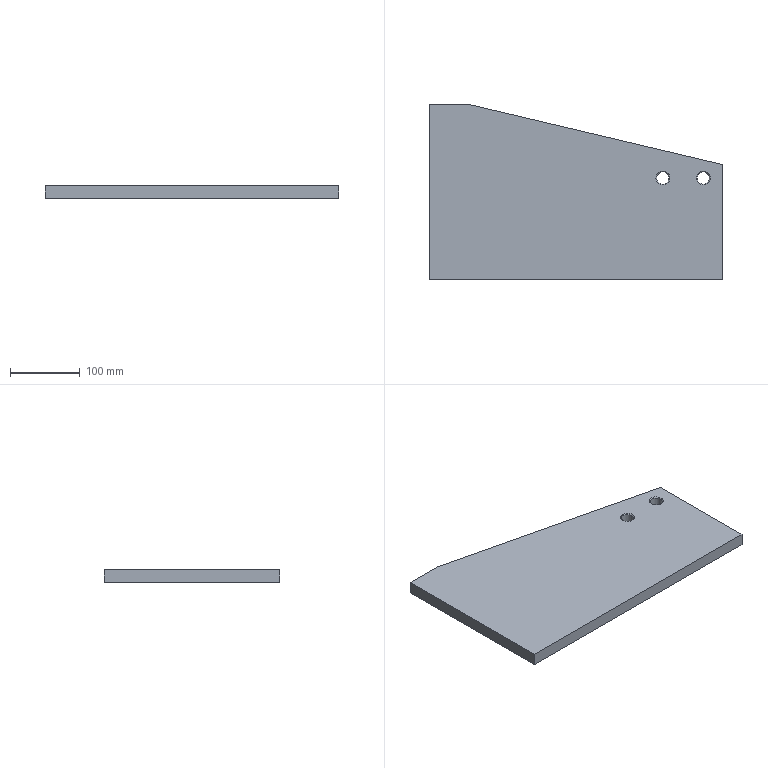Part | NX | features BREP 1 | 1 solid | 13 faces | box 421 x 252 x 18 mm | volume 1615279 mm3 | plane 7 | cone 4 | cylinder 2 | commonest cylinder face diameters 17.5 x2
STEP:
#1=CARTESIAN_POINT('',(-319.,-146.,-144.));
#2=VERTEX_POINT('',#1);
#3=CARTESIAN_POINT('',(-319.,106.,-144.));
#4=VERTEX_POINT('',#3);
#5=CARTESIAN_POINT('',(-319.,-146.,-144.));
#6=DIRECTION('',(0.,1.,0.));
#7=VECTOR('',#6,1000.);
#8=LINE('',#5,#7);
#9=EDGE_CURVE('',#2,#4,#8,.T.);
#10=ORIENTED_EDGE('',*,*,#9,.F.);
#11=CARTESIAN_POINT('',(-319.,-146.,-126.));
#12=VERTEX_POINT('',#11);
#13=CARTESIAN_POINT('',(-319.,-146.,-126.));
#14=DIRECTION('',(0.,0.,-1.));
#15=VECTOR('',#14,1000.);
#16=LINE('',#13,#15);
#17=EDGE_CURVE('',#12,#2,#16,.T.);
#18=ORIENTED_EDGE('',*,*,#17,.F.);
#19=CARTESIAN_POINT('',(-319.,106.,-126.));
#20=VERTEX_POINT('',#19);
#21=CARTESIAN_POINT('',(-319.,-146.,-126.));
#22=DIRECTION('',(0.,1.,0.));
#23=VECTOR('',#22,1000.);
#24=LINE('',#21,#23);
#25=EDGE_CURVE('',#12,#20,#24,.T.);
#26=ORIENTED_EDGE('',*,*,#25,.T.);
#27=CARTESIAN_POINT('',(-319.,106.,-126.));
#28=DIRECTION('',(0.,0.,-1.));
#29=VECTOR('',#28,1000.);
#30=LINE('',#27,#29);
#31=EDGE_CURVE('',#20,#4,#30,.T.);
#32=ORIENTED_EDGE('',*,*,#31,.T.);
#33=EDGE_LOOP('',(#10,#18,#26,#32));
#34=FACE_BOUND('',#33,.T.);
#35=CARTESIAN_POINT('',(-319.,-146.,-126.));
#36=DIRECTION('',(-1.,0.,0.));
#37=DIRECTION('',(0.,-1.,0.));
#38=AXIS2_PLACEMENT_3D('',#35,#36,#37);
#39=PLANE('',#38);
#40=ADVANCED_FACE('',(#34),#39,.T.);
#41=CARTESIAN_POINT('',(-264.,106.,-144.));
#42=VERTEX_POINT('',#41);
#43=CARTESIAN_POINT('',(-319.,106.,-144.));
#44=DIRECTION('',(1.,0.,0.));
#45=VECTOR('',#44,1000.);
#46=LINE('',#43,#45);
#47=EDGE_CURVE('',#4,#42,#46,.T.);
#48=ORIENTED_EDGE('',*,*,#47,.F.);
#49=ORIENTED_EDGE('',*,*,#31,.F.);
#50=CARTESIAN_POINT('',(-264.,106.,-126.));
#51=VERTEX_POINT('',#50);
#52=CARTESIAN_POINT('',(-319.,106.,-126.));
#53=DIRECTION('',(1.,0.,0.));
#54=VECTOR('',#53,1000.);
#55=LINE('',#52,#54);
#56=EDGE_CURVE('',#20,#51,#55,.T.);
#57=ORIENTED_EDGE('',*,*,#56,.T.);
#58=CARTESIAN_POINT('',(-264.,106.,-126.));
#59=DIRECTION('',(0.,0.,-1.));
#60=VECTOR('',#59,1000.);
#61=LINE('',#58,#60);
#62=EDGE_CURVE('',#51,#42,#61,.T.);
#63=ORIENTED_EDGE('',*,*,#62,.T.);
#64=EDGE_LOOP('',(#48,#49,#57,#63));
#65=FACE_BOUND('',#64,.T.);
#66=CARTESIAN_POINT('',(-319.,106.,-126.));
#67=DIRECTION('',(0.,1.,0.));
#68=DIRECTION('',(-1.,0.,0.));
#69=AXIS2_PLACEMENT_3D('',#66,#67,#68);
#70=PLANE('',#69);
#71=ADVANCED_FACE('',(#65),#70,.T.);
#72=CARTESIAN_POINT('',(102.,19.316,-144.));
#73=VERTEX_POINT('',#72);
#74=CARTESIAN_POINT('',(-264.,106.,-144.));
#75=DIRECTION('',(0.9731,-0.2305,0.));
#76=VECTOR('',#75,1000.);
#77=LINE('',#74,#76);
#78=EDGE_CURVE('',#42,#73,#77,.T.);
#79=ORIENTED_EDGE('',*,*,#78,.F.);
#80=ORIENTED_EDGE('',*,*,#62,.F.);
#81=CARTESIAN_POINT('',(102.,19.316,-126.));
#82=VERTEX_POINT('',#81);
#83=CARTESIAN_POINT('',(-264.,106.,-126.));
#84=DIRECTION('',(0.9731,-0.2305,0.));
#85=VECTOR('',#84,1000.);
#86=LINE('',#83,#85);
#87=EDGE_CURVE('',#51,#82,#86,.T.);
#88=ORIENTED_EDGE('',*,*,#87,.T.);
#89=CARTESIAN_POINT('',(102.,19.316,-126.));
#90=DIRECTION('',(0.,0.,-1.));
#91=VECTOR('',#90,1000.);
#92=LINE('',#89,#91);
#93=EDGE_CURVE('',#82,#73,#92,.T.);
#94=ORIENTED_EDGE('',*,*,#93,.T.);
#95=EDGE_LOOP('',(#79,#80,#88,#94));
#96=FACE_BOUND('',#95,.T.);
#97=CARTESIAN_POINT('',(-264.,106.,-126.));
#98=DIRECTION('',(0.2305,0.9731,0.));
#99=DIRECTION('',(-0.9731,0.2305,0.));
#100=AXIS2_PLACEMENT_3D('',#97,#98,#99);
#101=PLANE('',#100);
#102=ADVANCED_FACE('',(#96),#101,.T.);
#103=CARTESIAN_POINT('',(102.,-146.,-144.));
#104=VERTEX_POINT('',#103);
#105=CARTESIAN_POINT('',(102.,19.316,-144.));
#106=DIRECTION('',(0.,-1.,0.));
#107=VECTOR('',#106,1000.);
#108=LINE('',#105,#107);
#109=EDGE_CURVE('',#73,#104,#108,.T.);
#110=ORIENTED_EDGE('',*,*,#109,.F.);
#111=ORIENTED_EDGE('',*,*,#93,.F.);
#112=CARTESIAN_POINT('',(102.,-146.,-126.));
#113=VERTEX_POINT('',#112);
#114=CARTESIAN_POINT('',(102.,19.316,-126.));
#115=DIRECTION('',(0.,-1.,0.));
#116=VECTOR('',#115,1000.);
#117=LINE('',#114,#116);
#118=EDGE_CURVE('',#82,#113,#117,.T.);
#119=ORIENTED_EDGE('',*,*,#118,.T.);
#120=CARTESIAN_POINT('',(102.,-146.,-126.));
#121=DIRECTION('',(0.,0.,-1.));
#122=VECTOR('',#121,1000.);
#123=LINE('',#120,#122);
#124=EDGE_CURVE('',#113,#104,#123,.T.);
#125=ORIENTED_EDGE('',*,*,#124,.T.);
#126=EDGE_LOOP('',(#110,#111,#119,#125));
#127=FACE_BOUND('',#126,.T.);
#128=CARTESIAN_POINT('',(102.,19.316,-126.));
#129=DIRECTION('',(1.,0.,0.));
#130=DIRECTION('',(0.,1.,0.));
#131=AXIS2_PLACEMENT_3D('',#128,#129,#130);
#132=PLANE('',#131);
#133=ADVANCED_FACE('',(#127),#132,.T.);
#134=CARTESIAN_POINT('',(102.,-146.,-144.));
#135=DIRECTION('',(-1.,0.,0.));
#136=VECTOR('',#135,1000.);
#137=LINE('',#134,#136);
#138=EDGE_CURVE('',#104,#2,#137,.T.);
#139=ORIENTED_EDGE('',*,*,#138,.F.);
#140=ORIENTED_EDGE('',*,*,#124,.F.);
#141=CARTESIAN_POINT('',(102.,-146.,-126.));
#142=DIRECTION('',(-1.,0.,0.));
#143=VECTOR('',#142,1000.);
#144=LINE('',#141,#143);
#145=EDGE_CURVE('',#113,#12,#144,.T.);
#146=ORIENTED_EDGE('',*,*,#145,.T.);
#147=ORIENTED_EDGE('',*,*,#17,.T.);
#148=EDGE_LOOP('',(#139,#140,#146,#147));
#149=FACE_BOUND('',#148,.T.);
#150=CARTESIAN_POINT('',(102.,-146.,-126.));
#151=DIRECTION('',(0.,-1.,0.));
#152=DIRECTION('',(1.,0.,0.));
#153=AXIS2_PLACEMENT_3D('',#150,#151,#152);
#154=PLANE('',#153);
#155=ADVANCED_FACE('',(#149),#154,.T.);
#156=CARTESIAN_POINT('',(6.,0.,-126.));
#157=VERTEX_POINT('',#156);
#158=CARTESIAN_POINT('',(16.,0.,-126.));
#159=DIRECTION('',(0.,0.,-1.));
#160=DIRECTION('',(-1.,0.,0.));
#161=AXIS2_PLACEMENT_3D('',#158,#159,#160);
#162=CIRCLE('',#161,10.);
#163=EDGE_CURVE('',#157,#157,#162,.T.);
#164=ORIENTED_EDGE('',*,*,#163,.T.);
#165=EDGE_LOOP('',(#164));
#166=FACE_BOUND('',#165,.T.);
#167=CARTESIAN_POINT('',(64.,0.,-126.));
#168=VERTEX_POINT('',#167);
#169=CARTESIAN_POINT('',(74.,0.,-126.));
#170=DIRECTION('',(0.,0.,-1.));
#171=DIRECTION('',(-1.,0.,0.));
#172=AXIS2_PLACEMENT_3D('',#169,#170,#171);
#173=CIRCLE('',#172,10.);
#174=EDGE_CURVE('',#168,#168,#173,.T.);
#175=ORIENTED_EDGE('',*,*,#174,.T.);
#176=EDGE_LOOP('',(#175));
#177=FACE_BOUND('',#176,.T.);
#178=ORIENTED_EDGE('',*,*,#25,.F.);
#179=ORIENTED_EDGE('',*,*,#145,.F.);
#180=ORIENTED_EDGE('',*,*,#118,.F.);
#181=ORIENTED_EDGE('',*,*,#87,.F.);
#182=ORIENTED_EDGE('',*,*,#56,.F.);
#183=EDGE_LOOP('',(#178,#179,#180,#181,#182));
#184=FACE_BOUND('',#183,.T.);
#185=CARTESIAN_POINT('',(0.,0.,-126.));
#186=DIRECTION('',(0.,0.,-1.));
#187=DIRECTION('',(-1.,0.,0.));
#188=AXIS2_PLACEMENT_3D('',#185,#186,#187);
#189=PLANE('',#188);
#190=ADVANCED_FACE('',(#166,#177,#184),#189,.F.);
#191=CARTESIAN_POINT('',(6.,0.,-144.));
#192=VERTEX_POINT('',#191);
#193=CARTESIAN_POINT('',(16.,0.,-144.));
#194=DIRECTION('',(0.,0.,-1.));
#195=DIRECTION('',(-1.,0.,0.));
#196=AXIS2_PLACEMENT_3D('',#193,#194,#195);
#197=CIRCLE('',#196,10.);
#198=EDGE_CURVE('',#192,#192,#197,.F.);
#199=ORIENTED_EDGE('',*,*,#198,.T.);
#200=EDGE_LOOP('',(#199));
#201=FACE_BOUND('',#200,.T.);
#202=CARTESIAN_POINT('',(64.,0.,-144.));
#203=VERTEX_POINT('',#202);
#204=CARTESIAN_POINT('',(74.,0.,-144.));
#205=DIRECTION('',(0.,0.,-1.));
#206=DIRECTION('',(-1.,0.,0.));
#207=AXIS2_PLACEMENT_3D('',#204,#205,#206);
#208=CIRCLE('',#207,10.);
#209=EDGE_CURVE('',#203,#203,#208,.F.);
#210=ORIENTED_EDGE('',*,*,#209,.T.);
#211=EDGE_LOOP('',(#210));
#212=FACE_BOUND('',#211,.T.);
#213=ORIENTED_EDGE('',*,*,#9,.T.);
#214=ORIENTED_EDGE('',*,*,#47,.T.);
#215=ORIENTED_EDGE('',*,*,#78,.T.);
#216=ORIENTED_EDGE('',*,*,#109,.T.);
#217=ORIENTED_EDGE('',*,*,#138,.T.);
#218=EDGE_LOOP('',(#213,#214,#215,#216,#217));
#219=FACE_BOUND('',#218,.T.);
#220=CARTESIAN_POINT('',(0.,0.,-144.));
#221=DIRECTION('',(0.,0.,-1.));
#222=DIRECTION('',(-1.,0.,0.));
#223=AXIS2_PLACEMENT_3D('',#220,#221,#222);
#224=PLANE('',#223);
#225=ADVANCED_FACE('',(#201,#212,#219),#224,.T.);
#226=CARTESIAN_POINT('',(65.25,0.,-127.25));
#227=VERTEX_POINT('',#226);
#228=CARTESIAN_POINT('',(74.,0.,-127.25));
#229=DIRECTION('',(0.,0.,-1.));
#230=DIRECTION('',(-1.,0.,0.));
#231=AXIS2_PLACEMENT_3D('',#228,#229,#230);
#232=CIRCLE('',#231,8.75);
#233=EDGE_CURVE('',#227,#227,#232,.F.);
#234=ORIENTED_EDGE('',*,*,#233,.T.);
#235=EDGE_LOOP('',(#234));
#236=FACE_BOUND('',#235,.T.);
#237=CARTESIAN_POINT('',(65.25,0.,-142.75));
#238=VERTEX_POINT('',#237);
#239=CARTESIAN_POINT('',(74.,0.,-142.75));
#240=DIRECTION('',(0.,0.,-1.));
#241=DIRECTION('',(-1.,0.,0.));
#242=AXIS2_PLACEMENT_3D('',#239,#240,#241);
#243=CIRCLE('',#242,8.75);
#244=EDGE_CURVE('',#238,#238,#243,.T.);
#245=ORIENTED_EDGE('',*,*,#244,.T.);
#246=EDGE_LOOP('',(#245));
#247=FACE_BOUND('',#246,.T.);
#248=CARTESIAN_POINT('',(74.,0.,-144.));
#249=DIRECTION('',(0.,0.,1.));
#250=DIRECTION('',(1.,0.,0.));
#251=AXIS2_PLACEMENT_3D('',#248,#249,#250);
#252=CYLINDRICAL_SURFACE('',#251,8.75);
#253=ADVANCED_FACE('',(#236,#247),#252,.F.);
#254=ORIENTED_EDGE('',*,*,#244,.F.);
#255=EDGE_LOOP('',(#254));
#256=FACE_BOUND('',#255,.T.);
#257=ORIENTED_EDGE('',*,*,#209,.F.);
#258=EDGE_LOOP('',(#257));
#259=FACE_BOUND('',#258,.T.);
#260=CARTESIAN_POINT('',(74.,0.,-144.));
#261=DIRECTION('',(0.,0.,-1.));
#262=DIRECTION('',(-1.,0.,0.));
#263=AXIS2_PLACEMENT_3D('',#260,#261,#262);
#264=CONICAL_SURFACE('',#263,10.,0.7854);
#265=ADVANCED_FACE('',(#256,#259),#264,.F.);
#266=ORIENTED_EDGE('',*,*,#233,.F.);
#267=EDGE_LOOP('',(#266));
#268=FACE_BOUND('',#267,.T.);
#269=ORIENTED_EDGE('',*,*,#174,.F.);
#270=EDGE_LOOP('',(#269));
#271=FACE_BOUND('',#270,.T.);
#272=CARTESIAN_POINT('',(74.,0.,-126.));
#273=DIRECTION('',(0.,0.,1.));
#274=DIRECTION('',(1.,0.,0.));
#275=AXIS2_PLACEMENT_3D('',#272,#273,#274);
#276=CONICAL_SURFACE('',#275,10.,0.7854);
#277=ADVANCED_FACE('',(#268,#271),#276,.F.);
#278=CARTESIAN_POINT('',(7.25,0.,-127.25));
#279=VERTEX_POINT('',#278);
#280=CARTESIAN_POINT('',(16.,0.,-127.25));
#281=DIRECTION('',(0.,0.,-1.));
#282=DIRECTION('',(-1.,0.,0.));
#283=AXIS2_PLACEMENT_3D('',#280,#281,#282);
#284=CIRCLE('',#283,8.75);
#285=EDGE_CURVE('',#279,#279,#284,.F.);
#286=ORIENTED_EDGE('',*,*,#285,.T.);
#287=EDGE_LOOP('',(#286));
#288=FACE_BOUND('',#287,.T.);
#289=CARTESIAN_POINT('',(7.25,0.,-142.75));
#290=VERTEX_POINT('',#289);
#291=CARTESIAN_POINT('',(16.,0.,-142.75));
#292=DIRECTION('',(0.,0.,-1.));
#293=DIRECTION('',(-1.,0.,0.));
#294=AXIS2_PLACEMENT_3D('',#291,#292,#293);
#295=CIRCLE('',#294,8.75);
#296=EDGE_CURVE('',#290,#290,#295,.T.);
#297=ORIENTED_EDGE('',*,*,#296,.T.);
#298=EDGE_LOOP('',(#297));
#299=FACE_BOUND('',#298,.T.);
#300=CARTESIAN_POINT('',(16.,0.,-144.));
#301=DIRECTION('',(0.,0.,1.));
#302=DIRECTION('',(1.,0.,0.));
#303=AXIS2_PLACEMENT_3D('',#300,#301,#302);
#304=CYLINDRICAL_SURFACE('',#303,8.75);
#305=ADVANCED_FACE('',(#288,#299),#304,.F.);
#306=ORIENTED_EDGE('',*,*,#296,.F.);
#307=EDGE_LOOP('',(#306));
#308=FACE_BOUND('',#307,.T.);
#309=ORIENTED_EDGE('',*,*,#198,.F.);
#310=EDGE_LOOP('',(#309));
#311=FACE_BOUND('',#310,.T.);
#312=CARTESIAN_POINT('',(16.,0.,-144.));
#313=DIRECTION('',(0.,0.,-1.));
#314=DIRECTION('',(-1.,0.,0.));
#315=AXIS2_PLACEMENT_3D('',#312,#313,#314);
#316=CONICAL_SURFACE('',#315,10.,0.7854);
#317=ADVANCED_FACE('',(#308,#311),#316,.F.);
#318=ORIENTED_EDGE('',*,*,#285,.F.);
#319=EDGE_LOOP('',(#318));
#320=FACE_BOUND('',#319,.T.);
#321=ORIENTED_EDGE('',*,*,#163,.F.);
#322=EDGE_LOOP('',(#321));
#323=FACE_BOUND('',#322,.T.);
#324=CARTESIAN_POINT('',(16.,0.,-126.));
#325=DIRECTION('',(0.,0.,1.));
#326=DIRECTION('',(1.,0.,0.));
#327=AXIS2_PLACEMENT_3D('',#324,#325,#326);
#328=CONICAL_SURFACE('',#327,10.,0.7854);
#329=ADVANCED_FACE('',(#320,#323),#328,.F.);
#330=CLOSED_SHELL('',(#40,#71,#102,#133,#155,#190,#225,#253,#265,#277,#305,#317,#329));
#331=MANIFOLD_SOLID_BREP('',#330);
#332=(LENGTH_UNIT()NAMED_UNIT(*)SI_UNIT(.MILLI.,.METRE.));
#333=UNCERTAINTY_MEASURE_WITH_UNIT(LENGTH_MEASURE(0.00001),#332,'','');
#334=(NAMED_UNIT(*)PLANE_ANGLE_UNIT()SI_UNIT($,.RADIAN.));
#335=(NAMED_UNIT(*)SI_UNIT($,.STERADIAN.)SOLID_ANGLE_UNIT());
#336=(GEOMETRIC_REPRESENTATION_CONTEXT(3)GLOBAL_UNCERTAINTY_ASSIGNED_CONTEXT((#333))GLOBAL_UNIT_ASSIGNED_CONTEXT((#332,#334,#335))REPRESENTATION_CONTEXT('',''));
#337=ADVANCED_BREP_SHAPE_REPRESENTATION('',(#331),#336);